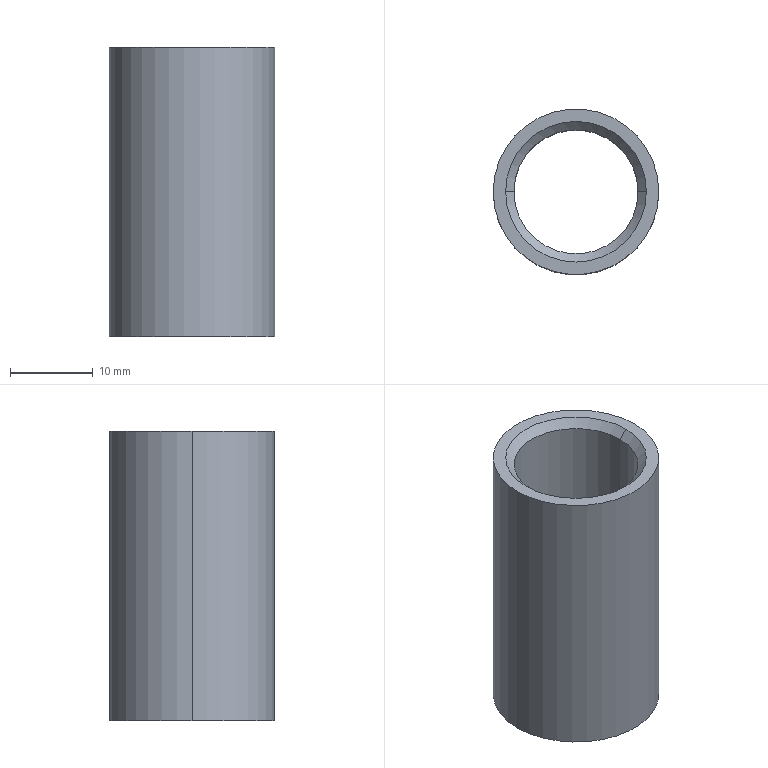Part | SolidWorks | features Chamfer 1, Extrusion 1 | 1 solid | 10 faces | box 20 x 20 x 35 mm | volume 4761 mm3 | cone 4 | cylinder 4 | plane 2 | commonest cylinder face diameters 15 x2 20 x2
STEP:
#1=CARTESIAN_POINT('',(-7.5,0.,34.));
#2=VERTEX_POINT('',#1);
#3=CARTESIAN_POINT('',(7.5,0.,34.));
#4=VERTEX_POINT('',#3);
#5=CARTESIAN_POINT('',(0.,0.,34.));
#6=DIRECTION('',(0.,0.,1.));
#7=DIRECTION('',(1.,0.,0.));
#8=AXIS2_PLACEMENT_3D('',#5,#6,#7);
#9=CIRCLE('',#8,7.5);
#10=EDGE_CURVE('',#2,#4,#9,.T.);
#11=ORIENTED_EDGE('',*,*,#10,.F.);
#12=CARTESIAN_POINT('',(-8.5,0.,35.));
#13=VERTEX_POINT('',#12);
#14=CARTESIAN_POINT('',(-7.5,0.,34.));
#15=DIRECTION('',(-0.7071,0.,0.7071));
#16=VECTOR('',#15,1000.);
#17=LINE('',#14,#16);
#18=EDGE_CURVE('',#2,#13,#17,.T.);
#19=ORIENTED_EDGE('',*,*,#18,.T.);
#20=CARTESIAN_POINT('',(8.5,0.,35.));
#21=VERTEX_POINT('',#20);
#22=CARTESIAN_POINT('',(0.,0.,35.));
#23=DIRECTION('',(0.,0.,-1.));
#24=DIRECTION('',(1.,0.,0.));
#25=AXIS2_PLACEMENT_3D('',#22,#23,#24);
#26=CIRCLE('',#25,8.5);
#27=EDGE_CURVE('',#21,#13,#26,.T.);
#28=ORIENTED_EDGE('',*,*,#27,.F.);
#29=CARTESIAN_POINT('',(7.5,0.,34.));
#30=DIRECTION('',(0.7071,0.,0.7071));
#31=VECTOR('',#30,1000.);
#32=LINE('',#29,#31);
#33=EDGE_CURVE('',#4,#21,#32,.T.);
#34=ORIENTED_EDGE('',*,*,#33,.F.);
#35=EDGE_LOOP('',(#11,#19,#28,#34));
#36=FACE_OUTER_BOUND('',#35,.T.);
#37=CARTESIAN_POINT('',(0.,0.,34.));
#38=DIRECTION('',(0.,0.,1.));
#39=DIRECTION('',(1.,0.,0.));
#40=AXIS2_PLACEMENT_3D('',#37,#38,#39);
#41=CONICAL_SURFACE('',#40,7.5,0.7854);
#42=ADVANCED_FACE('',(#36),#41,.F.);
#43=CARTESIAN_POINT('',(7.5,0.,1.));
#44=VERTEX_POINT('',#43);
#45=CARTESIAN_POINT('',(-7.5,0.,1.));
#46=VERTEX_POINT('',#45);
#47=CARTESIAN_POINT('',(0.,0.,1.));
#48=DIRECTION('',(0.,0.,-1.));
#49=DIRECTION('',(1.,0.,0.));
#50=AXIS2_PLACEMENT_3D('',#47,#48,#49);
#51=CIRCLE('',#50,7.5);
#52=EDGE_CURVE('',#44,#46,#51,.T.);
#53=ORIENTED_EDGE('',*,*,#52,.F.);
#54=CARTESIAN_POINT('',(8.5,0.,0.));
#55=VERTEX_POINT('',#54);
#56=CARTESIAN_POINT('',(8.5,0.,0.));
#57=DIRECTION('',(0.7071,0.,-0.7071));
#58=VECTOR('',#57,1000.);
#59=LINE('',#56,#58);
#60=EDGE_CURVE('',#44,#55,#59,.T.);
#61=ORIENTED_EDGE('',*,*,#60,.T.);
#62=CARTESIAN_POINT('',(-8.5,0.,0.));
#63=VERTEX_POINT('',#62);
#64=CARTESIAN_POINT('',(0.,0.,0.));
#65=DIRECTION('',(0.,0.,1.));
#66=DIRECTION('',(1.,0.,0.));
#67=AXIS2_PLACEMENT_3D('',#64,#65,#66);
#68=CIRCLE('',#67,8.5);
#69=EDGE_CURVE('',#63,#55,#68,.T.);
#70=ORIENTED_EDGE('',*,*,#69,.F.);
#71=CARTESIAN_POINT('',(-8.5,0.,0.));
#72=DIRECTION('',(-0.7071,0.,-0.7071));
#73=VECTOR('',#72,1000.);
#74=LINE('',#71,#73);
#75=EDGE_CURVE('',#46,#63,#74,.T.);
#76=ORIENTED_EDGE('',*,*,#75,.F.);
#77=EDGE_LOOP('',(#53,#61,#70,#76));
#78=FACE_OUTER_BOUND('',#77,.T.);
#79=CARTESIAN_POINT('',(0.,0.,0.));
#80=DIRECTION('',(0.,0.,-1.));
#81=DIRECTION('',(-1.,0.,0.));
#82=AXIS2_PLACEMENT_3D('',#79,#80,#81);
#83=CONICAL_SURFACE('',#82,8.5,0.7854);
#84=ADVANCED_FACE('',(#78),#83,.F.);
#85=ORIENTED_EDGE('',*,*,#10,.T.);
#86=CARTESIAN_POINT('',(7.5,0.,35.));
#87=DIRECTION('',(0.,0.,-1.));
#88=VECTOR('',#87,1000.);
#89=LINE('',#86,#88);
#90=EDGE_CURVE('',#4,#44,#89,.T.);
#91=ORIENTED_EDGE('',*,*,#90,.T.);
#92=ORIENTED_EDGE('',*,*,#52,.T.);
#93=CARTESIAN_POINT('',(-7.5,0.,35.));
#94=DIRECTION('',(0.,0.,-1.));
#95=VECTOR('',#94,1000.);
#96=LINE('',#93,#95);
#97=EDGE_CURVE('',#2,#46,#96,.T.);
#98=ORIENTED_EDGE('',*,*,#97,.F.);
#99=EDGE_LOOP('',(#85,#91,#92,#98));
#100=FACE_OUTER_BOUND('',#99,.T.);
#101=CARTESIAN_POINT('',(0.,0.,35.));
#102=DIRECTION('',(0.,0.,-1.));
#103=DIRECTION('',(-1.,0.,0.));
#104=AXIS2_PLACEMENT_3D('',#101,#102,#103);
#105=CYLINDRICAL_SURFACE('',#104,7.5);
#106=ADVANCED_FACE('',(#100),#105,.F.);
#107=CARTESIAN_POINT('',(10.,0.,35.));
#108=VERTEX_POINT('',#107);
#109=CARTESIAN_POINT('',(-10.,0.,35.));
#110=VERTEX_POINT('',#109);
#111=CARTESIAN_POINT('',(0.,0.,35.));
#112=DIRECTION('',(0.,0.,1.));
#113=DIRECTION('',(1.,0.,0.));
#114=AXIS2_PLACEMENT_3D('',#111,#112,#113);
#115=CIRCLE('',#114,10.);
#116=EDGE_CURVE('',#108,#110,#115,.T.);
#117=ORIENTED_EDGE('',*,*,#116,.F.);
#118=CARTESIAN_POINT('',(10.,0.,0.));
#119=VERTEX_POINT('',#118);
#120=CARTESIAN_POINT('',(10.,0.,35.));
#121=DIRECTION('',(0.,0.,-1.));
#122=VECTOR('',#121,1000.);
#123=LINE('',#120,#122);
#124=EDGE_CURVE('',#108,#119,#123,.T.);
#125=ORIENTED_EDGE('',*,*,#124,.T.);
#126=CARTESIAN_POINT('',(-10.,0.,0.));
#127=VERTEX_POINT('',#126);
#128=CARTESIAN_POINT('',(0.,0.,0.));
#129=DIRECTION('',(0.,0.,1.));
#130=DIRECTION('',(1.,0.,0.));
#131=AXIS2_PLACEMENT_3D('',#128,#129,#130);
#132=CIRCLE('',#131,10.);
#133=EDGE_CURVE('',#119,#127,#132,.T.);
#134=ORIENTED_EDGE('',*,*,#133,.T.);
#135=CARTESIAN_POINT('',(-10.,0.,35.));
#136=DIRECTION('',(0.,0.,-1.));
#137=VECTOR('',#136,1000.);
#138=LINE('',#135,#137);
#139=EDGE_CURVE('',#110,#127,#138,.T.);
#140=ORIENTED_EDGE('',*,*,#139,.F.);
#141=EDGE_LOOP('',(#117,#125,#134,#140));
#142=FACE_OUTER_BOUND('',#141,.T.);
#143=CARTESIAN_POINT('',(0.,0.,35.));
#144=DIRECTION('',(0.,0.,-1.));
#145=DIRECTION('',(-1.,0.,0.));
#146=AXIS2_PLACEMENT_3D('',#143,#144,#145);
#147=CYLINDRICAL_SURFACE('',#146,10.);
#148=ADVANCED_FACE('',(#142),#147,.T.);
#149=ORIENTED_EDGE('',*,*,#27,.T.);
#150=CARTESIAN_POINT('',(0.,0.,35.));
#151=DIRECTION('',(0.,0.,-1.));
#152=DIRECTION('',(1.,0.,0.));
#153=AXIS2_PLACEMENT_3D('',#150,#151,#152);
#154=CIRCLE('',#153,8.5);
#155=EDGE_CURVE('',#13,#21,#154,.T.);
#156=ORIENTED_EDGE('',*,*,#155,.T.);
#157=EDGE_LOOP('',(#149,#156));
#158=FACE_BOUND('',#157,.T.);
#159=CARTESIAN_POINT('',(0.,0.,35.));
#160=DIRECTION('',(0.,0.,1.));
#161=DIRECTION('',(1.,0.,0.));
#162=AXIS2_PLACEMENT_3D('',#159,#160,#161);
#163=CIRCLE('',#162,10.);
#164=EDGE_CURVE('',#110,#108,#163,.T.);
#165=ORIENTED_EDGE('',*,*,#164,.T.);
#166=ORIENTED_EDGE('',*,*,#116,.T.);
#167=EDGE_LOOP('',(#165,#166));
#168=FACE_OUTER_BOUND('',#167,.T.);
#169=CARTESIAN_POINT('',(0.,0.,35.));
#170=DIRECTION('',(0.,0.,1.));
#171=DIRECTION('',(1.,0.,0.));
#172=AXIS2_PLACEMENT_3D('',#169,#170,#171);
#173=PLANE('',#172);
#174=ADVANCED_FACE('',(#158,#168),#173,.T.);
#175=ORIENTED_EDGE('',*,*,#69,.T.);
#176=CARTESIAN_POINT('',(0.,0.,0.));
#177=DIRECTION('',(0.,0.,1.));
#178=DIRECTION('',(1.,0.,0.));
#179=AXIS2_PLACEMENT_3D('',#176,#177,#178);
#180=CIRCLE('',#179,8.5);
#181=EDGE_CURVE('',#55,#63,#180,.T.);
#182=ORIENTED_EDGE('',*,*,#181,.T.);
#183=EDGE_LOOP('',(#175,#182));
#184=FACE_BOUND('',#183,.T.);
#185=CARTESIAN_POINT('',(0.,0.,0.));
#186=DIRECTION('',(0.,0.,1.));
#187=DIRECTION('',(1.,0.,0.));
#188=AXIS2_PLACEMENT_3D('',#185,#186,#187);
#189=CIRCLE('',#188,10.);
#190=EDGE_CURVE('',#127,#119,#189,.T.);
#191=ORIENTED_EDGE('',*,*,#190,.F.);
#192=ORIENTED_EDGE('',*,*,#133,.F.);
#193=EDGE_LOOP('',(#191,#192));
#194=FACE_OUTER_BOUND('',#193,.T.);
#195=CARTESIAN_POINT('',(0.,0.,0.));
#196=DIRECTION('',(0.,0.,1.));
#197=DIRECTION('',(1.,0.,0.));
#198=AXIS2_PLACEMENT_3D('',#195,#196,#197);
#199=PLANE('',#198);
#200=ADVANCED_FACE('',(#184,#194),#199,.F.);
#201=ORIENTED_EDGE('',*,*,#124,.F.);
#202=ORIENTED_EDGE('',*,*,#164,.F.);
#203=ORIENTED_EDGE('',*,*,#139,.T.);
#204=ORIENTED_EDGE('',*,*,#190,.T.);
#205=EDGE_LOOP('',(#201,#202,#203,#204));
#206=FACE_OUTER_BOUND('',#205,.T.);
#207=CARTESIAN_POINT('',(0.,0.,35.));
#208=DIRECTION('',(0.,0.,-1.));
#209=DIRECTION('',(-1.,0.,0.));
#210=AXIS2_PLACEMENT_3D('',#207,#208,#209);
#211=CYLINDRICAL_SURFACE('',#210,10.);
#212=ADVANCED_FACE('',(#206),#211,.T.);
#213=ORIENTED_EDGE('',*,*,#90,.F.);
#214=CARTESIAN_POINT('',(0.,0.,34.));
#215=DIRECTION('',(0.,0.,1.));
#216=DIRECTION('',(1.,0.,0.));
#217=AXIS2_PLACEMENT_3D('',#214,#215,#216);
#218=CIRCLE('',#217,7.5);
#219=EDGE_CURVE('',#4,#2,#218,.T.);
#220=ORIENTED_EDGE('',*,*,#219,.T.);
#221=ORIENTED_EDGE('',*,*,#97,.T.);
#222=CARTESIAN_POINT('',(0.,0.,1.));
#223=DIRECTION('',(0.,0.,-1.));
#224=DIRECTION('',(1.,0.,0.));
#225=AXIS2_PLACEMENT_3D('',#222,#223,#224);
#226=CIRCLE('',#225,7.5);
#227=EDGE_CURVE('',#46,#44,#226,.T.);
#228=ORIENTED_EDGE('',*,*,#227,.T.);
#229=EDGE_LOOP('',(#213,#220,#221,#228));
#230=FACE_OUTER_BOUND('',#229,.T.);
#231=CARTESIAN_POINT('',(0.,0.,35.));
#232=DIRECTION('',(0.,0.,-1.));
#233=DIRECTION('',(-1.,0.,0.));
#234=AXIS2_PLACEMENT_3D('',#231,#232,#233);
#235=CYLINDRICAL_SURFACE('',#234,7.5);
#236=ADVANCED_FACE('',(#230),#235,.F.);
#237=ORIENTED_EDGE('',*,*,#60,.F.);
#238=ORIENTED_EDGE('',*,*,#227,.F.);
#239=ORIENTED_EDGE('',*,*,#75,.T.);
#240=ORIENTED_EDGE('',*,*,#181,.F.);
#241=EDGE_LOOP('',(#237,#238,#239,#240));
#242=FACE_OUTER_BOUND('',#241,.T.);
#243=CARTESIAN_POINT('',(0.,0.,0.));
#244=DIRECTION('',(0.,0.,-1.));
#245=DIRECTION('',(-1.,0.,0.));
#246=AXIS2_PLACEMENT_3D('',#243,#244,#245);
#247=CONICAL_SURFACE('',#246,8.5,0.7854);
#248=ADVANCED_FACE('',(#242),#247,.F.);
#249=ORIENTED_EDGE('',*,*,#18,.F.);
#250=ORIENTED_EDGE('',*,*,#219,.F.);
#251=ORIENTED_EDGE('',*,*,#33,.T.);
#252=ORIENTED_EDGE('',*,*,#155,.F.);
#253=EDGE_LOOP('',(#249,#250,#251,#252));
#254=FACE_OUTER_BOUND('',#253,.T.);
#255=CARTESIAN_POINT('',(0.,0.,34.));
#256=DIRECTION('',(0.,0.,1.));
#257=DIRECTION('',(1.,0.,0.));
#258=AXIS2_PLACEMENT_3D('',#255,#256,#257);
#259=CONICAL_SURFACE('',#258,7.5,0.7854);
#260=ADVANCED_FACE('',(#254),#259,.F.);
#261=CLOSED_SHELL('',(#42,#84,#106,#148,#174,#200,#212,#236,#248,#260));
#262=MANIFOLD_SOLID_BREP('',#261);
#263=CARTESIAN_POINT('',(0.,0.,0.));
#264=DIRECTION('',(0.,0.,1.));
#265=DIRECTION('',(1.,0.,0.));
#266=AXIS2_PLACEMENT_3D('',#263,#264,#265);
#267=(LENGTH_UNIT()NAMED_UNIT(*)SI_UNIT(.MILLI.,.METRE.));
#268=UNCERTAINTY_MEASURE_WITH_UNIT(LENGTH_MEASURE(0.00001),#267,'','');
#269=(NAMED_UNIT(*)PLANE_ANGLE_UNIT()SI_UNIT($,.RADIAN.));
#270=(NAMED_UNIT(*)SI_UNIT($,.STERADIAN.)SOLID_ANGLE_UNIT());
#271=(GEOMETRIC_REPRESENTATION_CONTEXT(3)GLOBAL_UNCERTAINTY_ASSIGNED_CONTEXT((#268))GLOBAL_UNIT_ASSIGNED_CONTEXT((#267,#269,#270))REPRESENTATION_CONTEXT('',''));
#272=ADVANCED_BREP_SHAPE_REPRESENTATION('',(#262,#266),#271);